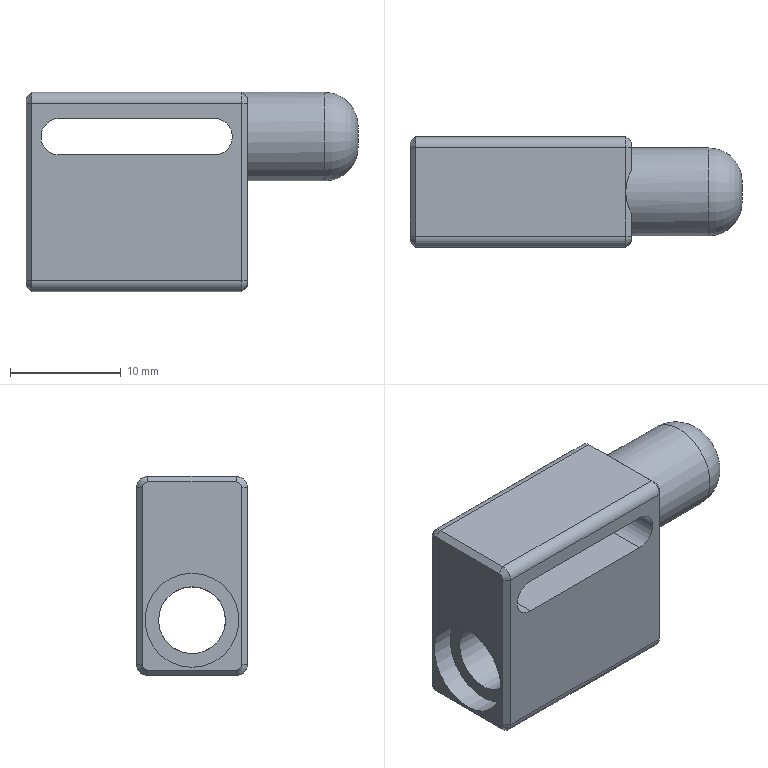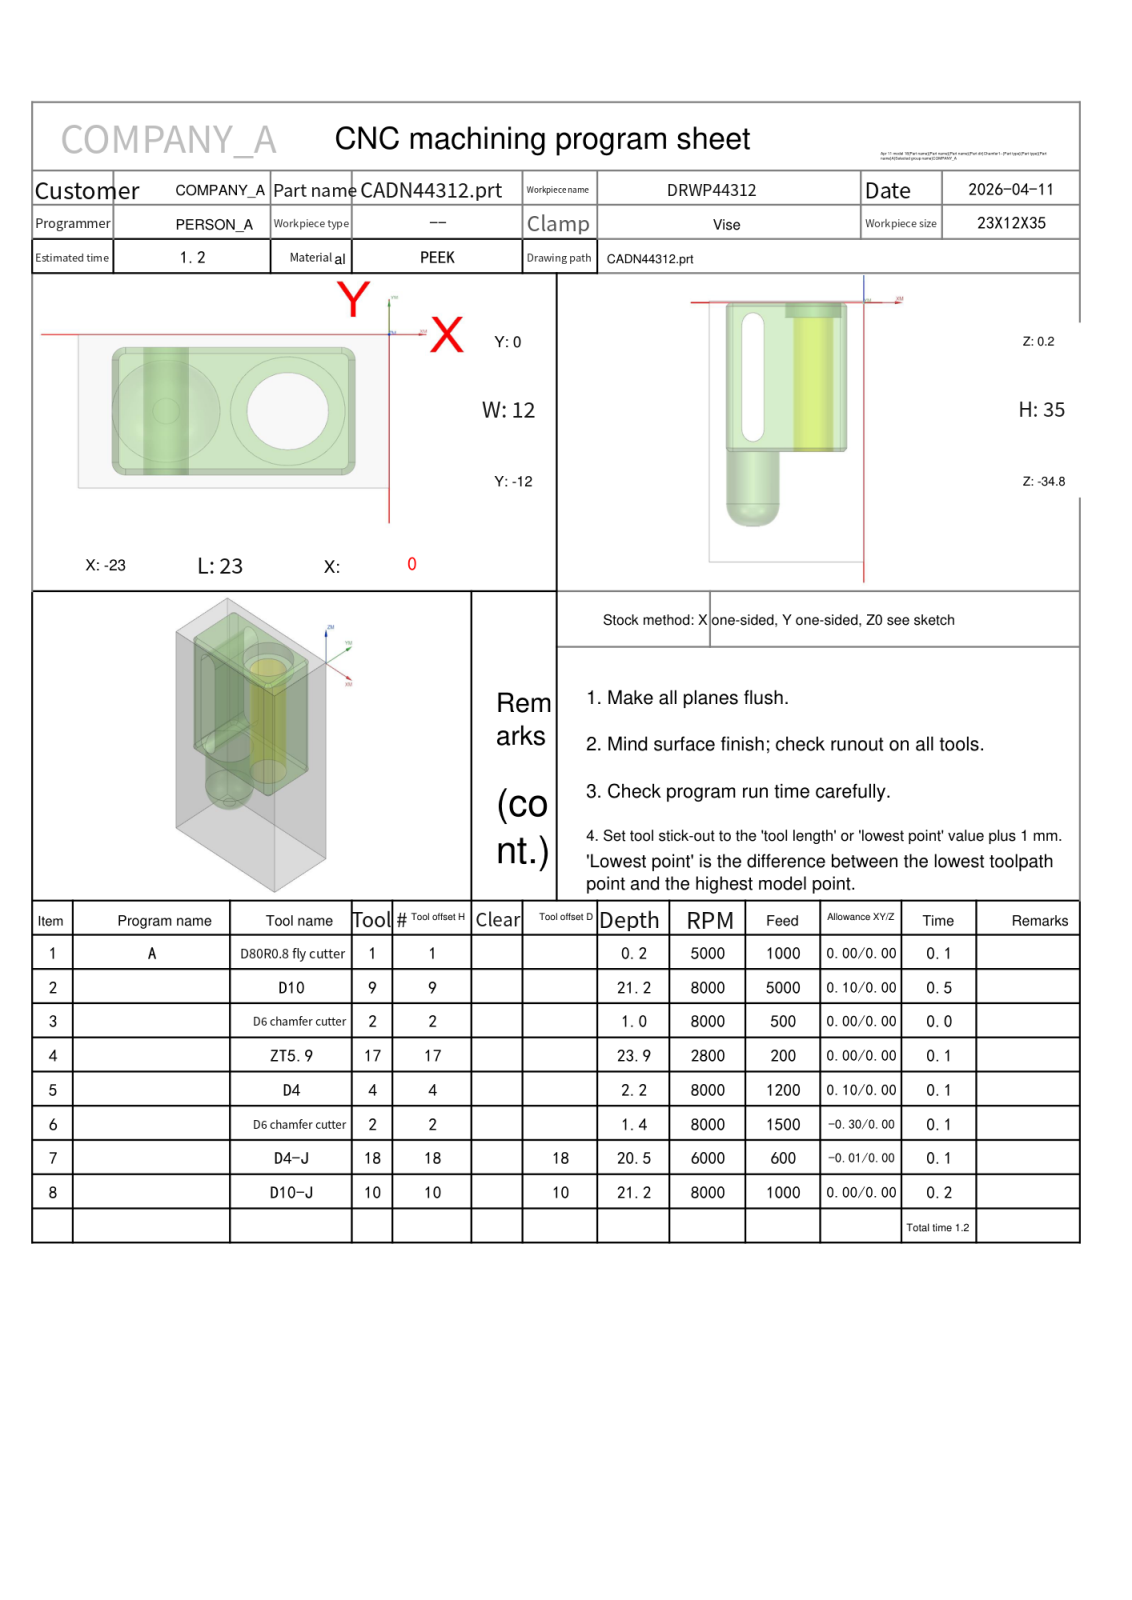NC program | NX | posted by the shop | part box 30 x 10 x 18 mm
Whole program:
%
O0001
(Machine time: 2.91 MIN)
(===Total Tool:7===)
(T1=D80R0.8 fly cutter  D=80.  R=0.8  D-  H01 Z=-0.   )
(T9=D10     D=10.  R=0.   D-  H09 Z=-21.  )
(T2=D6 chamfer cutter    D=6.   R=0.   D-  H02 Z=-1.2  )
(T17=ZT5.9  D=5.9  DR_a=120 D-  H17 Z=-23.7 )
(T4=D4      D=4.   R=0.   D-  H04 Z=-2.   )
(T18=D4-J   D=4.   R=0.   D18 H18 Z=-20.3 )
(T10=D10-J  D=10.  R=0.   D10 H10 Z=-21.  )
G80 G90 G17 G49 G40
G91 G28 Z0
M01
N1 T01 M06
(D80R0.8 fly cutter   D=80. R=0.8 H=01 ce=0.00 di=0.00)
G00 G90 G54 X42.5 Y-6. M03 S5000
G43 H01 Z20.
M08
Z2.
G01 Z0.0 F1000.
X37.5
X-60.5
X-65.5
Z2.
G00 Z20.
G91 G28 Z0.0
M05
M09
G91 G28 Z0.0
M01
N2 T09 M06
(D10  D=10. R=0. H=09 ce=0.10 di=0.00)
G00 G90 G54 X-11.5 Y4.1 M03 S8000
G43 H09 Z20.
M08
Z.5
G01 X-3.5 Z.426 F5000.
G02 X2.6 Y-2. Z.338 I0.0 J-6.1
G01 Y-10. Z.264
G02 X-3.5 Y-16.1 Z.176 I-6.1 J0.0
G01 X-19.5 Z.028
G02 X-25.6 Y-10. Z-.06 I0.0 J6.1
G01 Y-2. Z-.134
G02 X-19.5 Y4.1 Z-.223 I6.1 J0.0
G01 X-3.5 Z-.37
G02 X2.6 Y-2. Z-.458 I0.0 J-6.1
G01 Y-10. Z-.532
G02 X-3.5 Y-16.1 Z-.621 I-6.1 J0.0
G01 X-19.5 Z-.768
G02 X-25.6 Y-10. Z-.857 I0.0 J6.1
G01 Y-2. Z-.93
G02 X-19.5 Y4.1 Z-1.019 I6.1 J0.0
G01 X-3.5 Z-1.166
G02 X2.6 Y-2. Z-1.255 I0.0 J-6.1
G01 Y-10. Z-1.329
G02 X-3.5 Y-16.1 Z-1.417 I-6.1 J0.0
G01 X-19.5 Z-1.565
G02 X-25.6 Y-10. Z-1.653 I0.0 J6.1
G01 Y-2. Z-1.727
G02 X-19.5 Y4.1 Z-1.815 I6.1 J0.0
G01 X-3.5 Z-1.963
G02 X2.6 Y-2. Z-2.051 I0.0 J-6.1
G01 Y-10. Z-2.125
G02 X-3.5 Y-16.1 Z-2.213 I-6.1 J0.0
G01 X-19.5 Z-2.361
G02 X-25.6 Y-10. Z-2.449 I0.0 J6.1
G01 Y-2. Z-2.523
G02 X-19.5 Y4.1 Z-2.611 I6.1 J0.0
G01 X-3.5 Z-2.759
G02 X2.6 Y-2. Z-2.847 I0.0 J-6.1
G01 Y-10. Z-2.921
G02 X-3.5 Y-16.1 Z-3.01 I-6.1 J0.0
G01 X-19.5 Z-3.157
G02 X-25.6 Y-10. Z-3.246 I0.0 J6.1
G01 Y-2. Z-3.319
G02 X-19.5 Y4.1 Z-3.408 I6.1 J0.0
G01 X-3.5 Z-3.555
G02 X2.6 Y-2. Z-3.644 I0.0 J-6.1
G01 Y-10. Z-3.717
G02 X-3.5 Y-16.1 Z-3.806 I-6.1 J0.0
G01 X-19.5 Z-3.953
G02 X-25.6 Y-10. Z-4.042 I0.0 J6.1
G01 Y-2. Z-4.116
G02 X-19.5 Y4.1 Z-4.204 I6.1 J0.0
G01 X-3.5 Z-4.352
G02 X2.6 Y-2. Z-4.44 I0.0 J-6.1
G01 Y-10. Z-4.514
G02 X-3.5 Y-16.1 Z-4.602 I-6.1 J0.0
G01 X-19.5 Z-4.75
G02 X-25.6 Y-10. Z-4.838 I0.0 J6.1
G01 Y-2. Z-4.912
G02 X-19.5 Y4.1 Z-5. I6.1 J0.0
G01 X-3.5 Z-5.148
G02 X2.6 Y-2. Z-5.236 I0.0 J-6.1
G01 Y-10. Z-5.31
G02 X-3.5 Y-16.1 Z-5.398 I-6.1 J0.0
G01 X-19.5 Z-5.546
G02 X-25.6 Y-10. Z-5.634 I0.0 J6.1
G01 Y-2. Z-5.708
G02 X-19.5 Y4.1 Z-5.797 I6.1 J0.0
G01 X-3.5 Z-5.944
G02 X2.6 Y-2. Z-6.033 I0.0 J-6.1
G01 Y-10. Z-6.106
G02 X-3.5 Y-16.1 Z-6.195 I-6.1 J0.0
G01 X-19.5 Z-6.342
G02 X-25.6 Y-10. Z-6.431 I0.0 J6.1
G01 Y-2. Z-6.504
G02 X-19.5 Y4.1 Z-6.593 I6.1 J0.0
G01 X-3.5 Z-6.74
G02 X2.6 Y-2. Z-6.829 I0.0 J-6.1
G01 Y-10. Z-6.903
G02 X-3.5 Y-16.1 Z-6.991 I-6.1 J0.0
G01 X-19.5 Z-7.139
G02 X-25.6 Y-10. Z-7.227 I0.0 J6.1
G01 Y-2. Z-7.301
G02 X-19.5 Y4.1 Z-7.389 I6.1 J0.0
G01 X-3.5 Z-7.537
G02 X2.6 Y-2. Z-7.625 I0.0 J-6.1
G01 Y-10. Z-7.699
G02 X-3.5 Y-16.1 Z-7.787 I-6.1 J0.0
G01 X-19.5 Z-7.935
G02 X-25.6 Y-10. Z-8.023 I0.0 J6.1
G01 Y-2. Z-8.097
G02 X-19.5 Y4.1 Z-8.185 I6.1 J0.0
G01 X-3.5 Z-8.333
G02 X2.6 Y-2. Z-8.421 I0.0 J-6.1
G01 Y-10. Z-8.495
G02 X-3.5 Y-16.1 Z-8.584 I-6.1 J0.0
G01 X-19.5 Z-8.731
G02 X-25.6 Y-10. Z-8.82 I0.0 J6.1
G01 Y-2. Z-8.893
G02 X-19.5 Y4.1 Z-8.982 I6.1 J0.0
G01 X-3.5 Z-9.129
G02 X2.6 Y-2. Z-9.218 I0.0 J-6.1
G01 Y-10. Z-9.292
G02 X-3.5 Y-16.1 Z-9.38 I-6.1 J0.0
G01 X-19.5 Z-9.527
G02 X-25.6 Y-10. Z-9.616 I0.0 J6.1
G01 Y-2. Z-9.69
G02 X-19.5 Y4.1 Z-9.778 I6.1 J0.0
G01 X-3.5 Z-9.926
G02 X2.6 Y-2. Z-10.014 I0.0 J-6.1
G01 Y-10. Z-10.088
G02 X-3.5 Y-16.1 Z-10.176 I-6.1 J0.0
G01 X-19.5 Z-10.324
G02 X-25.6 Y-10. Z-10.412 I0.0 J6.1
G01 Y-2. Z-10.486
G02 X-19.5 Y4.1 Z-10.574 I6.1 J0.0
G01 X-3.5 Z-10.722
G02 X2.6 Y-2. Z-10.81 I0.0 J-6.1
G01 Y-10. Z-10.884
G02 X-3.5 Y-16.1 Z-10.973 I-6.1 J0.0
G01 X-19.5 Z-11.12
G02 X-25.6 Y-10. Z-11.208 I0.0 J6.1
G01 Y-2. Z-11.282
G02 X-19.5 Y4.1 Z-11.371 I6.1 J0.0
G01 X-3.5 Z-11.518
G02 X2.6 Y-2. Z-11.607 I0.0 J-6.1
G01 Y-10. Z-11.68
G02 X-3.5 Y-16.1 Z-11.769 I-6.1 J0.0
G01 X-19.5 Z-11.916
G02 X-25.6 Y-10. Z-12.005 I0.0 J6.1
G01 Y-2. Z-12.079
G02 X-19.5 Y4.1 Z-12.167 I6.1 J0.0
G01 X-3.5 Z-12.315
G02 X2.6 Y-2. Z-12.403 I0.0 J-6.1
G01 Y-10. Z-12.477
G02 X-3.5 Y-16.1 Z-12.565 I-6.1 J0.0
G01 X-19.5 Z-12.713
G02 X-25.6 Y-10. Z-12.801 I0.0 J6.1
G01 Y-2. Z-12.875
G02 X-19.5 Y4.1 Z-12.963 I6.1 J0.0
G01 X-3.5 Z-13.111
G02 X2.6 Y-2. Z-13.199 I0.0 J-6.1
G01 Y-10. Z-13.273
G02 X-3.5 Y-16.1 Z-13.361 I-6.1 J0.0
G01 X-19.5 Z-13.509
G02 X-25.6 Y-10. Z-13.597 I0.0 J6.1
G01 Y-2. Z-13.671
G02 X-19.5 Y4.1 Z-13.76 I6.1 J0.0
G01 X-3.5 Z-13.907
G02 X2.6 Y-2. Z-13.996 I0.0 J-6.1
G01 Y-10. Z-14.069
G02 X-3.5 Y-16.1 Z-14.158 I-6.1 J0.0
G01 X-19.5 Z-14.305
G02 X-25.6 Y-10. Z-14.394 I0.0 J6.1
G01 Y-2. Z-14.467
G02 X-19.5 Y4.1 Z-14.556 I6.1 J0.0
G01 X-3.5 Z-14.703
G02 X2.6 Y-2. Z-14.792 I0.0 J-6.1
G01 Y-10. Z-14.866
G02 X-3.5 Y-16.1 Z-14.954 I-6.1 J0.0
G01 X-19.5 Z-15.102
G02 X-25.6 Y-10. Z-15.19 I0.0 J6.1
G01 Y-2. Z-15.264
G02 X-19.5 Y4.1 Z-15.352 I6.1 J0.0
G01 X-3.5 Z-15.5
G02 X2.6 Y-2. Z-15.588 I0.0 J-6.1
G01 Y-10. Z-15.662
G02 X-3.5 Y-16.1 Z-15.75 I-6.1 J0.0
G01 X-19.5 Z-15.898
G02 X-25.6 Y-10. Z-15.986 I0.0 J6.1
G01 Y-2. Z-16.06
G02 X-19.5 Y4.1 Z-16.148 I6.1 J0.0
G01 X-3.5 Z-16.296
G02 X2.6 Y-2. Z-16.384 I0.0 J-6.1
G01 Y-10. Z-16.458
G02 X-3.5 Y-16.1 Z-16.547 I-6.1 J0.0
G01 X-19.5 Z-16.694
G02 X-25.6 Y-10. Z-16.783 I0.0 J6.1
G01 Y-2. Z-16.856
G02 X-19.5 Y4.1 Z-16.945 I6.1 J0.0
G01 X-3.5 Z-17.092
G02 X2.6 Y-2. Z-17.181 I0.0 J-6.1
G01 Y-10. Z-17.254
G02 X-3.5 Y-16.1 Z-17.343 I-6.1 J0.0
G01 X-19.5 Z-17.49
G02 X-25.6 Y-10. Z-17.579 I0.0 J6.1
G01 Y-2. Z-17.653
G02 X-19.5 Y4.1 Z-17.741 I6.1 J0.0
G01 X-3.5 Z-17.889
G02 X2.6 Y-2. Z-17.977 I0.0 J-6.1
G01 Y-10. Z-18.051
G02 X-3.5 Y-16.1 Z-18.139 I-6.1 J0.0
G01 X-19.5 Z-18.287
G02 X-25.6 Y-10. Z-18.375 I0.0 J6.1
G01 Y-2. Z-18.449
G02 X-19.5 Y4.1 Z-18.537 I6.1 J0.0
G01 X-3.5 Z-18.685
G02 X2.6 Y-2. Z-18.773 I0.0 J-6.1
G01 Y-10. Z-18.847
G02 X-3.5 Y-16.1 Z-18.935 I-6.1 J0.0
G01 X-19.5 Z-19.083
G02 X-25.6 Y-10. Z-19.171 I0.0 J6.1
G01 Y-2. Z-19.245
G02 X-19.5 Y4.1 Z-19.334 I6.1 J0.0
G01 X-3.5 Z-19.481
G02 X2.6 Y-2. Z-19.57 I0.0 J-6.1
G01 Y-10. Z-19.643
G02 X-3.5 Y-16.1 Z-19.732 I-6.1 J0.0
G01 X-19.5 Z-19.879
G02 X-25.6 Y-10. Z-19.968 I0.0 J6.1
G01 Y-2. Z-20.042
G02 X-19.5 Y4.1 Z-20.13 I6.1 J0.0
G01 X-3.5 Z-20.277
G02 X2.6 Y-2. Z-20.366 I0.0 J-6.1
G01 Y-10. Z-20.44
G02 X-3.5 Y-16.1 Z-20.528 I-6.1 J0.0
G01 X-19.5 Z-20.676
G02 X-25.6 Y-10. Z-20.764 I0.0 J6.1
G01 Y-2. Z-20.838
G02 X-19.5 Y4.1 Z-20.926 I6.1 J0.0
G01 X-11.5 Z-21.
X-3.5
G02 X2.6 Y-2. I0.0 J-6.1
G01 Y-10.
G02 X-3.5 Y-16.1 I-6.1 J0.0
G01 X-19.5
G02 X-25.6 Y-10. I0.0 J6.1
G01 Y-2.
G02 X-19.5 Y4.1 I6.1 J0.0
G01 X-11.5
X-11.
Z-20.
G00 Z20.
G91 G28 Z0.0
M05
M09
G91 G28 Z0.0
M01
N3 T02 M06
(D6 chamfer cutter   D=6. R=0. H=02 ce=0.00 di=0.00)
G00 G90 G54 X-7.5 Y-6. M03 S8000
G43 H02 Z20.
M08
G98 G81 X-7.5 Y-6. Z-.8 R1. F500.
G80
G00 Z20.
G91 G28 Z0.0
M05
M09
G91 G28 Z0.0
M01
N4 T17 M06
(ZT5.9 D=5.9 DR_a=120 H=17)
G00 G90 G54 X-7.5 Y-6. M03 S2800
G43 H17 Z20.
M08
G98 G83 X-7.5 Y-6. Z-23.703 R1. F200. Q2.
G80
G00 Z20.
G91 G28 Z0.0
M05
M09
G91 G28 Z0.0
M01
N5 T04 M06
(D4  D=4. R=0. H=04 ce=0.10 di=0.00)
G00 G90 G54 X-7.5 Y-6. M03 S8000
G43 H04 Z20.
M08
Z.5
G03 X-8.575 Y-7.075 I0.0 J-1.075 F1200.
X-7.5 Y-8.15 I1.075 J0.0
X-7.5 Y-8.15 Z.2 I0.0 J2.15
X-7.5 Y-8.15 Z-.1 I0.0 J2.15
X-7.5 Y-8.15 Z-.4 I0.0 J2.15
X-7.5 Y-8.15 Z-.7 I0.0 J2.15
X-7.5 Y-8.15 Z-1. I0.0 J2.15
X-7.5 Y-8.15 Z-1.3 I0.0 J2.15
X-7.5 Y-8.15 Z-1.6 I0.0 J2.15
X-7.5 Y-8.15 Z-1.9 I0.0 J2.15
X-5.638 Y-4.925 Z-2. I0.0 J2.15
X-7.5 Y-3.85 I-1.862 J-1.075
X-9.65 Y-6. I0.0 J-2.15
X-7.5 Y-8.15 I2.15 J0.0
X-5.35 Y-6. I0.0 J2.15
X-5.638 Y-4.925 I-2.15 J0.0
X-6.569 Y-4.388 I-.931 J-.538
X-7.644 Y-5.463 I0.0 J-1.075
X-7.5 Y-6. I1.075 J0.0
G00 Z20.
G91 G28 Z0.0
M05
M09
G91 G28 Z0.0
M01
N6 T02 M06
(D6 chamfer cutter   D=6. R=0. H=02 ce=-0.30 di=0.00)
G00 G90 G54 X-4.278 Y-4.508 M03 S8000
G43 H02 Z20.
M08
Z2.5
G01 X-4.296 Y-4.464 Z2.483 F500.
X-4.488 Y-4.116 Z2.338
X-4.717 Y-3.792 Z2.194
X-4.98 Y-3.495 Z2.049
X-5.276 Y-3.229 Z1.905
X-5.599 Y-2.999 Z1.76
X-5.851 Y-2.853 Z1.654
X-6.213 Y-2.688 Z1.509
X-6.59 Y-2.565 Z1.365
X-6.979 Y-2.485 Z1.22
X-7.374 Y-2.449 Z1.076
X-7.771 Y-2.457 Z.931
X-8.165 Y-2.51 Z.787
X-8.55 Y-2.606 Z.643
X-8.922 Y-2.744 Z.498
X-9.277 Y-2.923 Z.354
X-9.609 Y-3.14 Z.209
X-9.915 Y-3.393 Z.065
X-10.19 Y-3.679 Z-.08
X-10.432 Y-3.994 Z-.224
X-10.638 Y-4.333 Z-.369
X-10.804 Y-4.694 Z-.513
X-10.929 Y-5.071 Z-.658
X-11.012 Y-5.459 Z-.802
X-11.05 Y-5.854 Z-.947
Y-6. Z-1.
G03 X-7.5 Y-9.55 I3.55 J0.0
X-3.95 Y-6. I0.0 J3.55
X-7.5 Y-2.45 I-3.55 J0.0
X-11.05 Y-6. I0.0 J-3.55
X-11.015 Y-6.498 I3.55 J0.0
G01 Z1.5
G00 Z20.
G00 G90 X-20.674 Y.652 M03 S6500
Z20.
Z.3
G01 Z-1.2 F1500.
G03 X-19.5 Y-.3 I1.174 J.248
G01 X-3.5
G02 X-3.102 Y-.347 I0.0 J-1.7
G01 X-3.084 Y-.352
X-3.066 Y-.356
X-3.042 Y-.363
X-2.989 Y-.379
G02 X-1.8 Y-2. I-.511 J-1.621
G01 Y-10.
G02 X-3.5 Y-11.7 I-1.7 J0.0
G01 X-19.5
G02 X-21.2 Y-10. I0.0 J1.7
G01 Y-2.
G02 X-19.5 Y-.3 I1.7 J0.0
G01 X-19.1
G03 X-17.9 Y.9 I0.0 J1.2
G01 Z.3
G00 Z20.
G91 G28 Z0.0
M05
M09
G91 G28 Z0.0
M01
N7 T18 M06
(D4-J  D=4. R=0. H=18 ce=-0.01 di=0.00)
G00 G90 G54 X-6.473 Y-6.8 M03 S6000
G43 H18 Z10.2
M08
Z-1.
G01 Z-2. F600.
G41 D18
X-6.035
G03 X-5.235 Y-6. I0.0 J.8
X-7.5 Y-3.735 I-2.265 J0.0
X-9.765 Y-6. I0.0 J-2.265
X-7.5 Y-8.265 I2.265 J0.0
X-5.235 Y-6. I0.0 J2.265
X-5.27 Y-5.602 I-2.265 J0.0
X-6.058 Y-4.943 I-.788 J-.141
G01 X-6.198 Y-4.955
X-6.432 Y-4.997
G40 X-6.629 Y-5.032
Z-1.
G00 Z10.2
G00 G90 X-7.24 Y-6.355 M03 S6000
Z10.2
Z-5.075
G01 Z-6.575 F500.
G41 D18
X-7.06 Y-6.6
G03 X-6.46 Y-6. I0.0 J.6
X-7.5 Y-4.96 I-1.04 J0.0
X-8.54 Y-6. I0.0 J-1.04
X-7.5 Y-7.04 I1.04 J0.0
X-6.46 Y-6. I0.0 J1.04
X-6.536 Y-5.61 I-1.04 J0.0
X-7.092 Y-5.235 I-.556 J-.225
X-7.317 Y-5.279 I0.0 J-.6
G01 G40 X-7.392 Y-5.573
Z-5.075
G00 X-7.24 Y-6.355
Z-9.65
G01 Z-11.15
G41 D18
X-7.06 Y-6.6
G03 X-6.46 Y-6. I0.0 J.6
X-7.5 Y-4.96 I-1.04 J0.0
X-8.54 Y-6. I0.0 J-1.04
X-7.5 Y-7.04 I1.04 J0.0
X-6.46 Y-6. I0.0 J1.04
X-6.536 Y-5.61 I-1.04 J0.0
X-7.092 Y-5.235 I-.556 J-.225
X-7.317 Y-5.279 I0.0 J-.6
G01 G40 X-7.392 Y-5.573
Z-9.65
G00 X-7.24 Y-6.355
Z-14.225
G01 Z-15.725
G41 D18
X-7.06 Y-6.6
G03 X-6.46 Y-6. I0.0 J.6
X-7.5 Y-4.96 I-1.04 J0.0
X-8.54 Y-6. I0.0 J-1.04
X-7.5 Y-7.04 I1.04 J0.0
X-6.46 Y-6. I0.0 J1.04
X-6.536 Y-5.61 I-1.04 J0.0
X-7.092 Y-5.235 I-.556 J-.225
X-7.317 Y-5.279 I0.0 J-.6
G01 G40 X-7.392 Y-5.573
Z-14.225
G00 X-7.24 Y-6.355
Z-18.8
G01 Z-20.3
G41 D18
X-7.06 Y-6.6
G03 X-6.46 Y-6. I0.0 J.6
X-7.5 Y-4.96 I-1.04 J0.0
X-8.54 Y-6. I0.0 J-1.04
X-7.5 Y-7.04 I1.04 J0.0
X-6.46 Y-6. I0.0 J1.04
X-6.536 Y-5.61 I-1.04 J0.0
X-7.092 Y-5.235 I-.556 J-.225
X-7.317 Y-5.279 I0.0 J-.6
G01 G40 X-7.392 Y-5.573
Z-18.8
G00 Z10.2
G91 G28 Z0.0
M05
M09
G91 G28 Z0.0
M01
N8 T10 M06
(D10-J  D=10. R=0. H=10 ce=0.00 di=0.00)
G00 G90 G54 X-2.488 Y-17.128 M03 S8000
G43 H10 Z20.
M08
Z-10.
G01 Z-10.5 F1000.
G41 D10
X-2.503 Y-16.929
G03 X-3.5 Y-16. I-.997 J-.071
G01 X-19.5
G02 X-25.5 Y-10. I0.0 J6.
G01 Y-2.
G02 X-19.5 Y4. I6. J0.0
G01 X-3.5
G02 X2.5 Y-2. I0.0 J-6.
G01 Y-10.
G02 X-3.5 Y-16. I-6. J0.0
G01 X-4.
G03 X-5. Y-17. I0.0 J-1.
G01 G40 Y-17.2
Z-10.
G00 Z20.
X-2.488 Y-17.128
Z-20.5
G01 Z-21.
G41 D10
X-2.503 Y-16.929
G03 X-3.5 Y-16. I-.997 J-.071
G01 X-19.5
G02 X-25.5 Y-10. I0.0 J6.
G01 Y-2.
G02 X-19.5 Y4. I6. J0.0
G01 X-3.5
G02 X2.5 Y-2. I0.0 J-6.
G01 Y-10.
G02 X-3.5 Y-16. I-6. J0.0
G01 X-4.
G03 X-5. Y-17. I0.0 J-1.
G01 G40 Y-17.2
Z-20.5
G00 Z20.
M05
M09
G91 G28 Z0.0
G91 G28 Y0.0
M30
%